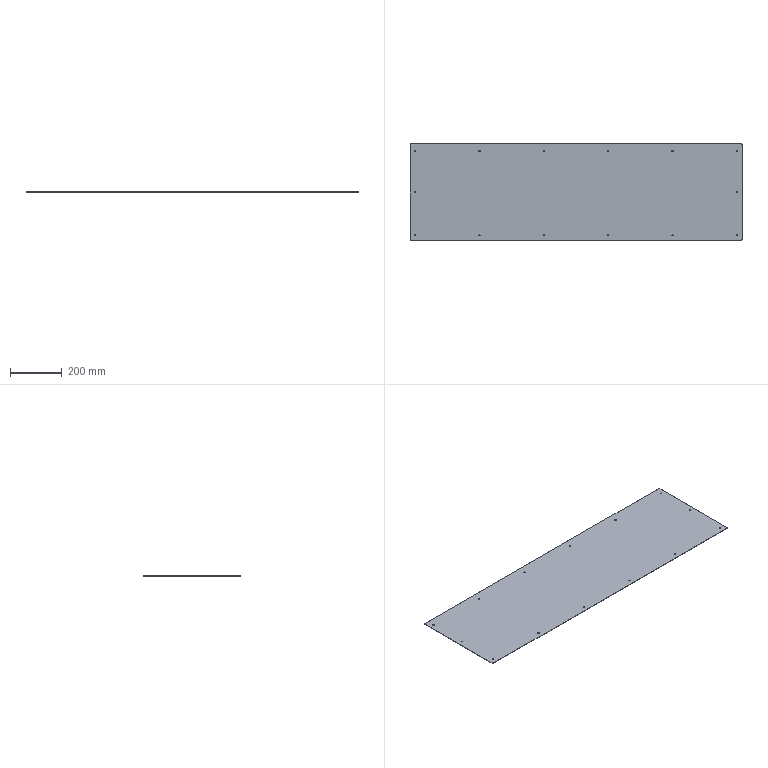Part | SolidWorks | features Fillet 1, FlatPattern 1, HoleWzd 1, SMBaseFlange 1, SheetMetal 1 | 1 solid | 38 faces | box 1280 x 374 x 1.5 mm | volume 717635 mm3 | cylinder 32 | plane 6 | commonest cylinder face diameters 5 x28 10 x4
STEP:
#1=CARTESIAN_POINT('',(-622.5,157.,-1.5));
#2=VERTEX_POINT('',#1);
#3=CARTESIAN_POINT('',(-617.5,157.,-1.5));
#4=VERTEX_POINT('',#3);
#5=CARTESIAN_POINT('',(-620.,157.,-1.5));
#6=DIRECTION('',(0.,0.,1.));
#7=DIRECTION('',(1.,0.,0.));
#8=AXIS2_PLACEMENT_3D('',#5,#6,#7);
#9=CIRCLE('',#8,2.5);
#10=EDGE_CURVE('',#2,#4,#9,.T.);
#11=ORIENTED_EDGE('',*,*,#10,.F.);
#12=CARTESIAN_POINT('',(-622.5,157.,0.));
#13=VERTEX_POINT('',#12);
#14=CARTESIAN_POINT('',(-622.5,157.,0.));
#15=DIRECTION('',(0.,0.,1.));
#16=VECTOR('',#15,1000.);
#17=LINE('',#14,#16);
#18=EDGE_CURVE('',#2,#13,#17,.T.);
#19=ORIENTED_EDGE('',*,*,#18,.T.);
#20=CARTESIAN_POINT('',(-617.5,157.,0.));
#21=VERTEX_POINT('',#20);
#22=CARTESIAN_POINT('',(-620.,157.,0.));
#23=DIRECTION('',(0.,0.,1.));
#24=DIRECTION('',(1.,0.,0.));
#25=AXIS2_PLACEMENT_3D('',#22,#23,#24);
#26=CIRCLE('',#25,2.5);
#27=EDGE_CURVE('',#13,#21,#26,.T.);
#28=ORIENTED_EDGE('',*,*,#27,.T.);
#29=CARTESIAN_POINT('',(-617.5,157.,0.));
#30=DIRECTION('',(0.,0.,1.));
#31=VECTOR('',#30,1000.);
#32=LINE('',#29,#31);
#33=EDGE_CURVE('',#4,#21,#32,.T.);
#34=ORIENTED_EDGE('',*,*,#33,.F.);
#35=EDGE_LOOP('',(#11,#19,#28,#34));
#36=FACE_OUTER_BOUND('',#35,.T.);
#37=CARTESIAN_POINT('',(-620.,157.,0.));
#38=DIRECTION('',(0.,0.,1.));
#39=DIRECTION('',(1.,0.,0.));
#40=AXIS2_PLACEMENT_3D('',#37,#38,#39);
#41=CYLINDRICAL_SURFACE('',#40,2.5);
#42=ADVANCED_FACE('',(#36),#41,.F.);
#43=CARTESIAN_POINT('',(617.5,157.,-1.5));
#44=VERTEX_POINT('',#43);
#45=CARTESIAN_POINT('',(622.5,157.,-1.5));
#46=VERTEX_POINT('',#45);
#47=CARTESIAN_POINT('',(620.,157.,-1.5));
#48=DIRECTION('',(0.,0.,1.));
#49=DIRECTION('',(1.,0.,0.));
#50=AXIS2_PLACEMENT_3D('',#47,#48,#49);
#51=CIRCLE('',#50,2.5);
#52=EDGE_CURVE('',#44,#46,#51,.T.);
#53=ORIENTED_EDGE('',*,*,#52,.F.);
#54=CARTESIAN_POINT('',(617.5,157.,0.));
#55=VERTEX_POINT('',#54);
#56=CARTESIAN_POINT('',(617.5,157.,0.));
#57=DIRECTION('',(0.,0.,1.));
#58=VECTOR('',#57,1000.);
#59=LINE('',#56,#58);
#60=EDGE_CURVE('',#44,#55,#59,.T.);
#61=ORIENTED_EDGE('',*,*,#60,.T.);
#62=CARTESIAN_POINT('',(622.5,157.,0.));
#63=VERTEX_POINT('',#62);
#64=CARTESIAN_POINT('',(620.,157.,0.));
#65=DIRECTION('',(0.,0.,1.));
#66=DIRECTION('',(1.,0.,0.));
#67=AXIS2_PLACEMENT_3D('',#64,#65,#66);
#68=CIRCLE('',#67,2.5);
#69=EDGE_CURVE('',#55,#63,#68,.T.);
#70=ORIENTED_EDGE('',*,*,#69,.T.);
#71=CARTESIAN_POINT('',(622.5,157.,0.));
#72=DIRECTION('',(0.,0.,1.));
#73=VECTOR('',#72,1000.);
#74=LINE('',#71,#73);
#75=EDGE_CURVE('',#46,#63,#74,.T.);
#76=ORIENTED_EDGE('',*,*,#75,.F.);
#77=EDGE_LOOP('',(#53,#61,#70,#76));
#78=FACE_OUTER_BOUND('',#77,.T.);
#79=CARTESIAN_POINT('',(620.,157.,0.));
#80=DIRECTION('',(0.,0.,1.));
#81=DIRECTION('',(1.,0.,0.));
#82=AXIS2_PLACEMENT_3D('',#79,#80,#81);
#83=CYLINDRICAL_SURFACE('',#82,2.5);
#84=ADVANCED_FACE('',(#78),#83,.F.);
#85=CARTESIAN_POINT('',(617.5,-167.,-1.5));
#86=VERTEX_POINT('',#85);
#87=CARTESIAN_POINT('',(622.5,-167.,-1.5));
#88=VERTEX_POINT('',#87);
#89=CARTESIAN_POINT('',(620.,-167.,-1.5));
#90=DIRECTION('',(0.,0.,1.));
#91=DIRECTION('',(1.,0.,0.));
#92=AXIS2_PLACEMENT_3D('',#89,#90,#91);
#93=CIRCLE('',#92,2.5);
#94=EDGE_CURVE('',#86,#88,#93,.T.);
#95=ORIENTED_EDGE('',*,*,#94,.F.);
#96=CARTESIAN_POINT('',(617.5,-167.,0.));
#97=VERTEX_POINT('',#96);
#98=CARTESIAN_POINT('',(617.5,-167.,0.));
#99=DIRECTION('',(0.,0.,1.));
#100=VECTOR('',#99,1000.);
#101=LINE('',#98,#100);
#102=EDGE_CURVE('',#86,#97,#101,.T.);
#103=ORIENTED_EDGE('',*,*,#102,.T.);
#104=CARTESIAN_POINT('',(622.5,-167.,0.));
#105=VERTEX_POINT('',#104);
#106=CARTESIAN_POINT('',(620.,-167.,0.));
#107=DIRECTION('',(0.,0.,1.));
#108=DIRECTION('',(1.,0.,0.));
#109=AXIS2_PLACEMENT_3D('',#106,#107,#108);
#110=CIRCLE('',#109,2.5);
#111=EDGE_CURVE('',#97,#105,#110,.T.);
#112=ORIENTED_EDGE('',*,*,#111,.T.);
#113=CARTESIAN_POINT('',(622.5,-167.,0.));
#114=DIRECTION('',(0.,0.,1.));
#115=VECTOR('',#114,1000.);
#116=LINE('',#113,#115);
#117=EDGE_CURVE('',#88,#105,#116,.T.);
#118=ORIENTED_EDGE('',*,*,#117,.F.);
#119=EDGE_LOOP('',(#95,#103,#112,#118));
#120=FACE_OUTER_BOUND('',#119,.T.);
#121=CARTESIAN_POINT('',(620.,-167.,0.));
#122=DIRECTION('',(0.,0.,1.));
#123=DIRECTION('',(1.,0.,0.));
#124=AXIS2_PLACEMENT_3D('',#121,#122,#123);
#125=CYLINDRICAL_SURFACE('',#124,2.5);
#126=ADVANCED_FACE('',(#120),#125,.F.);
#127=CARTESIAN_POINT('',(369.5,-167.,-1.5));
#128=VERTEX_POINT('',#127);
#129=CARTESIAN_POINT('',(374.5,-167.,-1.5));
#130=VERTEX_POINT('',#129);
#131=CARTESIAN_POINT('',(372.,-167.,-1.5));
#132=DIRECTION('',(0.,0.,1.));
#133=DIRECTION('',(1.,0.,0.));
#134=AXIS2_PLACEMENT_3D('',#131,#132,#133);
#135=CIRCLE('',#134,2.5);
#136=EDGE_CURVE('',#128,#130,#135,.T.);
#137=ORIENTED_EDGE('',*,*,#136,.F.);
#138=CARTESIAN_POINT('',(369.5,-167.,0.));
#139=VERTEX_POINT('',#138);
#140=CARTESIAN_POINT('',(369.5,-167.,0.));
#141=DIRECTION('',(0.,0.,1.));
#142=VECTOR('',#141,1000.);
#143=LINE('',#140,#142);
#144=EDGE_CURVE('',#128,#139,#143,.T.);
#145=ORIENTED_EDGE('',*,*,#144,.T.);
#146=CARTESIAN_POINT('',(374.5,-167.,0.));
#147=VERTEX_POINT('',#146);
#148=CARTESIAN_POINT('',(372.,-167.,0.));
#149=DIRECTION('',(0.,0.,1.));
#150=DIRECTION('',(1.,0.,0.));
#151=AXIS2_PLACEMENT_3D('',#148,#149,#150);
#152=CIRCLE('',#151,2.5);
#153=EDGE_CURVE('',#139,#147,#152,.T.);
#154=ORIENTED_EDGE('',*,*,#153,.T.);
#155=CARTESIAN_POINT('',(374.5,-167.,0.));
#156=DIRECTION('',(0.,0.,1.));
#157=VECTOR('',#156,1000.);
#158=LINE('',#155,#157);
#159=EDGE_CURVE('',#130,#147,#158,.T.);
#160=ORIENTED_EDGE('',*,*,#159,.F.);
#161=EDGE_LOOP('',(#137,#145,#154,#160));
#162=FACE_OUTER_BOUND('',#161,.T.);
#163=CARTESIAN_POINT('',(372.,-167.,0.));
#164=DIRECTION('',(0.,0.,1.));
#165=DIRECTION('',(1.,0.,0.));
#166=AXIS2_PLACEMENT_3D('',#163,#164,#165);
#167=CYLINDRICAL_SURFACE('',#166,2.5);
#168=ADVANCED_FACE('',(#162),#167,.F.);
#169=CARTESIAN_POINT('',(-374.5,-167.,-1.5));
#170=VERTEX_POINT('',#169);
#171=CARTESIAN_POINT('',(-369.5,-167.,-1.5));
#172=VERTEX_POINT('',#171);
#173=CARTESIAN_POINT('',(-372.,-167.,-1.5));
#174=DIRECTION('',(0.,0.,1.));
#175=DIRECTION('',(1.,0.,0.));
#176=AXIS2_PLACEMENT_3D('',#173,#174,#175);
#177=CIRCLE('',#176,2.5);
#178=EDGE_CURVE('',#170,#172,#177,.T.);
#179=ORIENTED_EDGE('',*,*,#178,.F.);
#180=CARTESIAN_POINT('',(-374.5,-167.,0.));
#181=VERTEX_POINT('',#180);
#182=CARTESIAN_POINT('',(-374.5,-167.,0.));
#183=DIRECTION('',(0.,0.,1.));
#184=VECTOR('',#183,1000.);
#185=LINE('',#182,#184);
#186=EDGE_CURVE('',#170,#181,#185,.T.);
#187=ORIENTED_EDGE('',*,*,#186,.T.);
#188=CARTESIAN_POINT('',(-369.5,-167.,0.));
#189=VERTEX_POINT('',#188);
#190=CARTESIAN_POINT('',(-372.,-167.,0.));
#191=DIRECTION('',(0.,0.,1.));
#192=DIRECTION('',(1.,0.,0.));
#193=AXIS2_PLACEMENT_3D('',#190,#191,#192);
#194=CIRCLE('',#193,2.5);
#195=EDGE_CURVE('',#181,#189,#194,.T.);
#196=ORIENTED_EDGE('',*,*,#195,.T.);
#197=CARTESIAN_POINT('',(-369.5,-167.,0.));
#198=DIRECTION('',(0.,0.,1.));
#199=VECTOR('',#198,1000.);
#200=LINE('',#197,#199);
#201=EDGE_CURVE('',#172,#189,#200,.T.);
#202=ORIENTED_EDGE('',*,*,#201,.F.);
#203=EDGE_LOOP('',(#179,#187,#196,#202));
#204=FACE_OUTER_BOUND('',#203,.T.);
#205=CARTESIAN_POINT('',(-372.,-167.,0.));
#206=DIRECTION('',(0.,0.,1.));
#207=DIRECTION('',(1.,0.,0.));
#208=AXIS2_PLACEMENT_3D('',#205,#206,#207);
#209=CYLINDRICAL_SURFACE('',#208,2.5);
#210=ADVANCED_FACE('',(#204),#209,.F.);
#211=CARTESIAN_POINT('',(-622.5,0.,-1.5));
#212=VERTEX_POINT('',#211);
#213=CARTESIAN_POINT('',(-617.5,0.,-1.5));
#214=VERTEX_POINT('',#213);
#215=CARTESIAN_POINT('',(-620.,0.,-1.5));
#216=DIRECTION('',(0.,0.,1.));
#217=DIRECTION('',(1.,0.,0.));
#218=AXIS2_PLACEMENT_3D('',#215,#216,#217);
#219=CIRCLE('',#218,2.5);
#220=EDGE_CURVE('',#212,#214,#219,.T.);
#221=ORIENTED_EDGE('',*,*,#220,.F.);
#222=CARTESIAN_POINT('',(-622.5,0.,0.));
#223=VERTEX_POINT('',#222);
#224=CARTESIAN_POINT('',(-622.5,0.,0.));
#225=DIRECTION('',(0.,0.,1.));
#226=VECTOR('',#225,1000.);
#227=LINE('',#224,#226);
#228=EDGE_CURVE('',#212,#223,#227,.T.);
#229=ORIENTED_EDGE('',*,*,#228,.T.);
#230=CARTESIAN_POINT('',(-617.5,0.,0.));
#231=VERTEX_POINT('',#230);
#232=CARTESIAN_POINT('',(-620.,0.,0.));
#233=DIRECTION('',(0.,0.,1.));
#234=DIRECTION('',(1.,0.,0.));
#235=AXIS2_PLACEMENT_3D('',#232,#233,#234);
#236=CIRCLE('',#235,2.5);
#237=EDGE_CURVE('',#223,#231,#236,.T.);
#238=ORIENTED_EDGE('',*,*,#237,.T.);
#239=CARTESIAN_POINT('',(-617.5,0.,0.));
#240=DIRECTION('',(0.,0.,1.));
#241=VECTOR('',#240,1000.);
#242=LINE('',#239,#241);
#243=EDGE_CURVE('',#214,#231,#242,.T.);
#244=ORIENTED_EDGE('',*,*,#243,.F.);
#245=EDGE_LOOP('',(#221,#229,#238,#244));
#246=FACE_OUTER_BOUND('',#245,.T.);
#247=CARTESIAN_POINT('',(-620.,0.,0.));
#248=DIRECTION('',(0.,0.,1.));
#249=DIRECTION('',(1.,0.,0.));
#250=AXIS2_PLACEMENT_3D('',#247,#248,#249);
#251=CYLINDRICAL_SURFACE('',#250,2.5);
#252=ADVANCED_FACE('',(#246),#251,.F.);
#253=CARTESIAN_POINT('',(-622.5,-167.,-1.5));
#254=VERTEX_POINT('',#253);
#255=CARTESIAN_POINT('',(-617.5,-167.,-1.5));
#256=VERTEX_POINT('',#255);
#257=CARTESIAN_POINT('',(-620.,-167.,-1.5));
#258=DIRECTION('',(0.,0.,1.));
#259=DIRECTION('',(1.,0.,0.));
#260=AXIS2_PLACEMENT_3D('',#257,#258,#259);
#261=CIRCLE('',#260,2.5);
#262=EDGE_CURVE('',#254,#256,#261,.T.);
#263=ORIENTED_EDGE('',*,*,#262,.F.);
#264=CARTESIAN_POINT('',(-622.5,-167.,0.));
#265=VERTEX_POINT('',#264);
#266=CARTESIAN_POINT('',(-622.5,-167.,0.));
#267=DIRECTION('',(0.,0.,1.));
#268=VECTOR('',#267,1000.);
#269=LINE('',#266,#268);
#270=EDGE_CURVE('',#254,#265,#269,.T.);
#271=ORIENTED_EDGE('',*,*,#270,.T.);
#272=CARTESIAN_POINT('',(-617.5,-167.,0.));
#273=VERTEX_POINT('',#272);
#274=CARTESIAN_POINT('',(-620.,-167.,0.));
#275=DIRECTION('',(0.,0.,1.));
#276=DIRECTION('',(1.,0.,0.));
#277=AXIS2_PLACEMENT_3D('',#274,#275,#276);
#278=CIRCLE('',#277,2.5);
#279=EDGE_CURVE('',#265,#273,#278,.T.);
#280=ORIENTED_EDGE('',*,*,#279,.T.);
#281=CARTESIAN_POINT('',(-617.5,-167.,0.));
#282=DIRECTION('',(0.,0.,1.));
#283=VECTOR('',#282,1000.);
#284=LINE('',#281,#283);
#285=EDGE_CURVE('',#256,#273,#284,.T.);
#286=ORIENTED_EDGE('',*,*,#285,.F.);
#287=EDGE_LOOP('',(#263,#271,#280,#286));
#288=FACE_OUTER_BOUND('',#287,.T.);
#289=CARTESIAN_POINT('',(-620.,-167.,0.));
#290=DIRECTION('',(0.,0.,1.));
#291=DIRECTION('',(1.,0.,0.));
#292=AXIS2_PLACEMENT_3D('',#289,#290,#291);
#293=CYLINDRICAL_SURFACE('',#292,2.5);
#294=ADVANCED_FACE('',(#288),#293,.F.);
#295=CARTESIAN_POINT('',(617.5,0.,-1.5));
#296=VERTEX_POINT('',#295);
#297=CARTESIAN_POINT('',(622.5,0.,-1.5));
#298=VERTEX_POINT('',#297);
#299=CARTESIAN_POINT('',(620.,0.,-1.5));
#300=DIRECTION('',(0.,0.,1.));
#301=DIRECTION('',(1.,0.,0.));
#302=AXIS2_PLACEMENT_3D('',#299,#300,#301);
#303=CIRCLE('',#302,2.5);
#304=EDGE_CURVE('',#296,#298,#303,.T.);
#305=ORIENTED_EDGE('',*,*,#304,.F.);
#306=CARTESIAN_POINT('',(617.5,0.,0.));
#307=VERTEX_POINT('',#306);
#308=CARTESIAN_POINT('',(617.5,0.,0.));
#309=DIRECTION('',(0.,0.,1.));
#310=VECTOR('',#309,1000.);
#311=LINE('',#308,#310);
#312=EDGE_CURVE('',#296,#307,#311,.T.);
#313=ORIENTED_EDGE('',*,*,#312,.T.);
#314=CARTESIAN_POINT('',(622.5,0.,0.));
#315=VERTEX_POINT('',#314);
#316=CARTESIAN_POINT('',(620.,0.,0.));
#317=DIRECTION('',(0.,0.,1.));
#318=DIRECTION('',(1.,0.,0.));
#319=AXIS2_PLACEMENT_3D('',#316,#317,#318);
#320=CIRCLE('',#319,2.5);
#321=EDGE_CURVE('',#307,#315,#320,.T.);
#322=ORIENTED_EDGE('',*,*,#321,.T.);
#323=CARTESIAN_POINT('',(622.5,0.,0.));
#324=DIRECTION('',(0.,0.,1.));
#325=VECTOR('',#324,1000.);
#326=LINE('',#323,#325);
#327=EDGE_CURVE('',#298,#315,#326,.T.);
#328=ORIENTED_EDGE('',*,*,#327,.F.);
#329=EDGE_LOOP('',(#305,#313,#322,#328));
#330=FACE_OUTER_BOUND('',#329,.T.);
#331=CARTESIAN_POINT('',(620.,0.,0.));
#332=DIRECTION('',(0.,0.,1.));
#333=DIRECTION('',(1.,0.,0.));
#334=AXIS2_PLACEMENT_3D('',#331,#332,#333);
#335=CYLINDRICAL_SURFACE('',#334,2.5);
#336=ADVANCED_FACE('',(#330),#335,.F.);
#337=CARTESIAN_POINT('',(-126.5,-167.,-1.5));
#338=VERTEX_POINT('',#337);
#339=CARTESIAN_POINT('',(-121.5,-167.,-1.5));
#340=VERTEX_POINT('',#339);
#341=CARTESIAN_POINT('',(-124.,-167.,-1.5));
#342=DIRECTION('',(0.,0.,1.));
#343=DIRECTION('',(1.,0.,0.));
#344=AXIS2_PLACEMENT_3D('',#341,#342,#343);
#345=CIRCLE('',#344,2.5);
#346=EDGE_CURVE('',#338,#340,#345,.T.);
#347=ORIENTED_EDGE('',*,*,#346,.F.);
#348=CARTESIAN_POINT('',(-126.5,-167.,0.));
#349=VERTEX_POINT('',#348);
#350=CARTESIAN_POINT('',(-126.5,-167.,0.));
#351=DIRECTION('',(0.,0.,1.));
#352=VECTOR('',#351,1000.);
#353=LINE('',#350,#352);
#354=EDGE_CURVE('',#338,#349,#353,.T.);
#355=ORIENTED_EDGE('',*,*,#354,.T.);
#356=CARTESIAN_POINT('',(-121.5,-167.,0.));
#357=VERTEX_POINT('',#356);
#358=CARTESIAN_POINT('',(-124.,-167.,0.));
#359=DIRECTION('',(0.,0.,1.));
#360=DIRECTION('',(1.,0.,0.));
#361=AXIS2_PLACEMENT_3D('',#358,#359,#360);
#362=CIRCLE('',#361,2.5);
#363=EDGE_CURVE('',#349,#357,#362,.T.);
#364=ORIENTED_EDGE('',*,*,#363,.T.);
#365=CARTESIAN_POINT('',(-121.5,-167.,0.));
#366=DIRECTION('',(0.,0.,1.));
#367=VECTOR('',#366,1000.);
#368=LINE('',#365,#367);
#369=EDGE_CURVE('',#340,#357,#368,.T.);
#370=ORIENTED_EDGE('',*,*,#369,.F.);
#371=EDGE_LOOP('',(#347,#355,#364,#370));
#372=FACE_OUTER_BOUND('',#371,.T.);
#373=CARTESIAN_POINT('',(-124.,-167.,0.));
#374=DIRECTION('',(0.,0.,1.));
#375=DIRECTION('',(1.,0.,0.));
#376=AXIS2_PLACEMENT_3D('',#373,#374,#375);
#377=CYLINDRICAL_SURFACE('',#376,2.5);
#378=ADVANCED_FACE('',(#372),#377,.F.);
#379=CARTESIAN_POINT('',(121.5,-167.,-1.5));
#380=VERTEX_POINT('',#379);
#381=CARTESIAN_POINT('',(126.5,-167.,-1.5));
#382=VERTEX_POINT('',#381);
#383=CARTESIAN_POINT('',(124.,-167.,-1.5));
#384=DIRECTION('',(0.,0.,1.));
#385=DIRECTION('',(1.,0.,0.));
#386=AXIS2_PLACEMENT_3D('',#383,#384,#385);
#387=CIRCLE('',#386,2.5);
#388=EDGE_CURVE('',#380,#382,#387,.T.);
#389=ORIENTED_EDGE('',*,*,#388,.F.);
#390=CARTESIAN_POINT('',(121.5,-167.,0.));
#391=VERTEX_POINT('',#390);
#392=CARTESIAN_POINT('',(121.5,-167.,0.));
#393=DIRECTION('',(0.,0.,1.));
#394=VECTOR('',#393,1000.);
#395=LINE('',#392,#394);
#396=EDGE_CURVE('',#380,#391,#395,.T.);
#397=ORIENTED_EDGE('',*,*,#396,.T.);
#398=CARTESIAN_POINT('',(126.5,-167.,0.));
#399=VERTEX_POINT('',#398);
#400=CARTESIAN_POINT('',(124.,-167.,0.));
#401=DIRECTION('',(0.,0.,1.));
#402=DIRECTION('',(1.,0.,0.));
#403=AXIS2_PLACEMENT_3D('',#400,#401,#402);
#404=CIRCLE('',#403,2.5);
#405=EDGE_CURVE('',#391,#399,#404,.T.);
#406=ORIENTED_EDGE('',*,*,#405,.T.);
#407=CARTESIAN_POINT('',(126.5,-167.,0.));
#408=DIRECTION('',(0.,0.,1.));
#409=VECTOR('',#408,1000.);
#410=LINE('',#407,#409);
#411=EDGE_CURVE('',#382,#399,#410,.T.);
#412=ORIENTED_EDGE('',*,*,#411,.F.);
#413=EDGE_LOOP('',(#389,#397,#406,#412));
#414=FACE_OUTER_BOUND('',#413,.T.);
#415=CARTESIAN_POINT('',(124.,-167.,0.));
#416=DIRECTION('',(0.,0.,1.));
#417=DIRECTION('',(1.,0.,0.));
#418=AXIS2_PLACEMENT_3D('',#415,#416,#417);
#419=CYLINDRICAL_SURFACE('',#418,2.5);
#420=ADVANCED_FACE('',(#414),#419,.F.);
#421=CARTESIAN_POINT('',(-126.5,157.,-1.5));
#422=VERTEX_POINT('',#421);
#423=CARTESIAN_POINT('',(-121.5,157.,-1.5));
#424=VERTEX_POINT('',#423);
#425=CARTESIAN_POINT('',(-124.,157.,-1.5));
#426=DIRECTION('',(0.,0.,1.));
#427=DIRECTION('',(1.,0.,0.));
#428=AXIS2_PLACEMENT_3D('',#425,#426,#427);
#429=CIRCLE('',#428,2.5);
#430=EDGE_CURVE('',#422,#424,#429,.T.);
#431=ORIENTED_EDGE('',*,*,#430,.F.);
#432=CARTESIAN_POINT('',(-126.5,157.,0.));
#433=VERTEX_POINT('',#432);
#434=CARTESIAN_POINT('',(-126.5,157.,0.));
#435=DIRECTION('',(0.,0.,1.));
#436=VECTOR('',#435,1000.);
#437=LINE('',#434,#436);
#438=EDGE_CURVE('',#422,#433,#437,.T.);
#439=ORIENTED_EDGE('',*,*,#438,.T.);
#440=CARTESIAN_POINT('',(-121.5,157.,0.));
#441=VERTEX_POINT('',#440);
#442=CARTESIAN_POINT('',(-124.,157.,0.));
#443=DIRECTION('',(0.,0.,1.));
#444=DIRECTION('',(1.,0.,0.));
#445=AXIS2_PLACEMENT_3D('',#442,#443,#444);
#446=CIRCLE('',#445,2.5);
#447=EDGE_CURVE('',#433,#441,#446,.T.);
#448=ORIENTED_EDGE('',*,*,#447,.T.);
#449=CARTESIAN_POINT('',(-121.5,157.,0.));
#450=DIRECTION('',(0.,0.,1.));
#451=VECTOR('',#450,1000.);
#452=LINE('',#449,#451);
#453=EDGE_CURVE('',#424,#441,#452,.T.);
#454=ORIENTED_EDGE('',*,*,#453,.F.);
#455=EDGE_LOOP('',(#431,#439,#448,#454));
#456=FACE_OUTER_BOUND('',#455,.T.);
#457=CARTESIAN_POINT('',(-124.,157.,0.));
#458=DIRECTION('',(0.,0.,1.));
#459=DIRECTION('',(1.,0.,0.));
#460=AXIS2_PLACEMENT_3D('',#457,#458,#459);
#461=CYLINDRICAL_SURFACE('',#460,2.5);
#462=ADVANCED_FACE('',(#456),#461,.F.);
#463=CARTESIAN_POINT('',(121.5,157.,-1.5));
#464=VERTEX_POINT('',#463);
#465=CARTESIAN_POINT('',(126.5,157.,-1.5));
#466=VERTEX_POINT('',#465);
#467=CARTESIAN_POINT('',(124.,157.,-1.5));
#468=DIRECTION('',(0.,0.,1.));
#469=DIRECTION('',(1.,0.,0.));
#470=AXIS2_PLACEMENT_3D('',#467,#468,#469);
#471=CIRCLE('',#470,2.5);
#472=EDGE_CURVE('',#464,#466,#471,.T.);
#473=ORIENTED_EDGE('',*,*,#472,.F.);
#474=CARTESIAN_POINT('',(121.5,157.,0.));
#475=VERTEX_POINT('',#474);
#476=CARTESIAN_POINT('',(121.5,157.,0.));
#477=DIRECTION('',(0.,0.,1.));
#478=VECTOR('',#477,1000.);
#479=LINE('',#476,#478);
#480=EDGE_CURVE('',#464,#475,#479,.T.);
#481=ORIENTED_EDGE('',*,*,#480,.T.);
#482=CARTESIAN_POINT('',(126.5,157.,0.));
#483=VERTEX_POINT('',#482);
#484=CARTESIAN_POINT('',(124.,157.,0.));
#485=DIRECTION('',(0.,0.,1.));
#486=DIRECTION('',(1.,0.,0.));
#487=AXIS2_PLACEMENT_3D('',#484,#485,#486);
#488=CIRCLE('',#487,2.5);
#489=EDGE_CURVE('',#475,#483,#488,.T.);
#490=ORIENTED_EDGE('',*,*,#489,.T.);
#491=CARTESIAN_POINT('',(126.5,157.,0.));
#492=DIRECTION('',(0.,0.,1.));
#493=VECTOR('',#492,1000.);
#494=LINE('',#491,#493);
#495=EDGE_CURVE('',#466,#483,#494,.T.);
#496=ORIENTED_EDGE('',*,*,#495,.F.);
#497=EDGE_LOOP('',(#473,#481,#490,#496));
#498=FACE_OUTER_BOUND('',#497,.T.);
#499=CARTESIAN_POINT('',(124.,157.,0.));
#500=DIRECTION('',(0.,0.,1.));
#501=DIRECTION('',(1.,0.,0.));
#502=AXIS2_PLACEMENT_3D('',#499,#500,#501);
#503=CYLINDRICAL_SURFACE('',#502,2.5);
#504=ADVANCED_FACE('',(#498),#503,.F.);
#505=CARTESIAN_POINT('',(369.5,157.,-1.5));
#506=VERTEX_POINT('',#505);
#507=CARTESIAN_POINT('',(374.5,157.,-1.5));
#508=VERTEX_POINT('',#507);
#509=CARTESIAN_POINT('',(372.,157.,-1.5));
#510=DIRECTION('',(0.,0.,1.));
#511=DIRECTION('',(1.,0.,0.));
#512=AXIS2_PLACEMENT_3D('',#509,#510,#511);
#513=CIRCLE('',#512,2.5);
#514=EDGE_CURVE('',#506,#508,#513,.T.);
#515=ORIENTED_EDGE('',*,*,#514,.F.);
#516=CARTESIAN_POINT('',(369.5,157.,0.));
#517=VERTEX_POINT('',#516);
#518=CARTESIAN_POINT('',(369.5,157.,0.));
#519=DIRECTION('',(0.,0.,1.));
#520=VECTOR('',#519,1000.);
#521=LINE('',#518,#520);
#522=EDGE_CURVE('',#506,#517,#521,.T.);
#523=ORIENTED_EDGE('',*,*,#522,.T.);
#524=CARTESIAN_POINT('',(374.5,157.,0.));
#525=VERTEX_POINT('',#524);
#526=CARTESIAN_POINT('',(372.,157.,0.));
#527=DIRECTION('',(0.,0.,1.));
#528=DIRECTION('',(1.,0.,0.));
#529=AXIS2_PLACEMENT_3D('',#526,#527,#528);
#530=CIRCLE('',#529,2.5);
#531=EDGE_CURVE('',#517,#525,#530,.T.);
#532=ORIENTED_EDGE('',*,*,#531,.T.);
#533=CARTESIAN_POINT('',(374.5,157.,0.));
#534=DIRECTION('',(0.,0.,1.));
#535=VECTOR('',#534,1000.);
#536=LINE('',#533,#535);
#537=EDGE_CURVE('',#508,#525,#536,.T.);
#538=ORIENTED_EDGE('',*,*,#537,.F.);
#539=EDGE_LOOP('',(#515,#523,#532,#538));
#540=FACE_OUTER_BOUND('',#539,.T.);
#541=CARTESIAN_POINT('',(372.,157.,0.));
#542=DIRECTION('',(0.,0.,1.));
#543=DIRECTION('',(1.,0.,0.));
#544=AXIS2_PLACEMENT_3D('',#541,#542,#543);
#545=CYLINDRICAL_SURFACE('',#544,2.5);
#546=ADVANCED_FACE('',(#540),#545,.F.);
#547=CARTESIAN_POINT('',(-374.5,157.,-1.5));
#548=VERTEX_POINT('',#547);
#549=CARTESIAN_POINT('',(-369.5,157.,-1.5));
#550=VERTEX_POINT('',#549);
#551=CARTESIAN_POINT('',(-372.,157.,-1.5));
#552=DIRECTION('',(0.,0.,1.));
#553=DIRECTION('',(1.,0.,0.));
#554=AXIS2_PLACEMENT_3D('',#551,#552,#553);
#555=CIRCLE('',#554,2.5);
#556=EDGE_CURVE('',#548,#550,#555,.T.);
#557=ORIENTED_EDGE('',*,*,#556,.F.);
#558=CARTESIAN_POINT('',(-374.5,157.,0.));
#559=VERTEX_POINT('',#558);
#560=CARTESIAN_POINT('',(-374.5,157.,0.));
#561=DIRECTION('',(0.,0.,1.));
#562=VECTOR('',#561,1000.);
#563=LINE('',#560,#562);
#564=EDGE_CURVE('',#548,#559,#563,.T.);
#565=ORIENTED_EDGE('',*,*,#564,.T.);
#566=CARTESIAN_POINT('',(-369.5,157.,0.));
#567=VERTEX_POINT('',#566);
#568=CARTESIAN_POINT('',(-372.,157.,0.));
#569=DIRECTION('',(0.,0.,1.));
#570=DIRECTION('',(1.,0.,0.));
#571=AXIS2_PLACEMENT_3D('',#568,#569,#570);
#572=CIRCLE('',#571,2.5);
#573=EDGE_CURVE('',#559,#567,#572,.T.);
#574=ORIENTED_EDGE('',*,*,#573,.T.);
#575=CARTESIAN_POINT('',(-369.5,157.,0.));
#576=DIRECTION('',(0.,0.,1.));
#577=VECTOR('',#576,1000.);
#578=LINE('',#575,#577);
#579=EDGE_CURVE('',#550,#567,#578,.T.);
#580=ORIENTED_EDGE('',*,*,#579,.F.);
#581=EDGE_LOOP('',(#557,#565,#574,#580));
#582=FACE_OUTER_BOUND('',#581,.T.);
#583=CARTESIAN_POINT('',(-372.,157.,0.));
#584=DIRECTION('',(0.,0.,1.));
#585=DIRECTION('',(1.,0.,0.));
#586=AXIS2_PLACEMENT_3D('',#583,#584,#585);
#587=CYLINDRICAL_SURFACE('',#586,2.5);
#588=ADVANCED_FACE('',(#582),#587,.F.);
#589=CARTESIAN_POINT('',(640.,-182.,0.));
#590=VERTEX_POINT('',#589);
#591=CARTESIAN_POINT('',(640.,182.,0.));
#592=VERTEX_POINT('',#591);
#593=CARTESIAN_POINT('',(640.,187.,0.));
#594=DIRECTION('',(0.,1.,0.));
#595=VECTOR('',#594,1000.);
#596=LINE('',#593,#595);
#597=EDGE_CURVE('',#590,#592,#596,.T.);
#598=ORIENTED_EDGE('',*,*,#597,.F.);
#599=CARTESIAN_POINT('',(640.,-182.,-1.5));
#600=VERTEX_POINT('',#599);
#601=CARTESIAN_POINT('',(640.,-182.,-1.5));
#602=DIRECTION('',(0.,0.,-1.));
#603=VECTOR('',#602,1000.);
#604=LINE('',#601,#603);
#605=EDGE_CURVE('',#590,#600,#604,.T.);
#606=ORIENTED_EDGE('',*,*,#605,.T.);
#607=CARTESIAN_POINT('',(640.,182.,-1.5));
#608=VERTEX_POINT('',#607);
#609=CARTESIAN_POINT('',(640.,187.,-1.5));
#610=DIRECTION('',(0.,1.,0.));
#611=VECTOR('',#610,1000.);
#612=LINE('',#609,#611);
#613=EDGE_CURVE('',#600,#608,#612,.T.);
#614=ORIENTED_EDGE('',*,*,#613,.T.);
#615=CARTESIAN_POINT('',(640.,182.,-1.5));
#616=DIRECTION('',(0.,0.,1.));
#617=VECTOR('',#616,1000.);
#618=LINE('',#615,#617);
#619=EDGE_CURVE('',#608,#592,#618,.T.);
#620=ORIENTED_EDGE('',*,*,#619,.T.);
#621=EDGE_LOOP('',(#598,#606,#614,#620));
#622=FACE_OUTER_BOUND('',#621,.T.);
#623=CARTESIAN_POINT('',(640.,187.,-1.5));
#624=DIRECTION('',(1.,0.,0.));
#625=DIRECTION('',(0.,0.,-1.));
#626=AXIS2_PLACEMENT_3D('',#623,#624,#625);
#627=PLANE('',#626);
#628=ADVANCED_FACE('',(#622),#627,.T.);
#629=CARTESIAN_POINT('',(-635.,-187.,0.));
#630=VERTEX_POINT('',#629);
#631=CARTESIAN_POINT('',(635.,-187.,0.));
#632=VERTEX_POINT('',#631);
#633=CARTESIAN_POINT('',(-640.,-187.,0.));
#634=DIRECTION('',(1.,0.,0.));
#635=VECTOR('',#634,1000.);
#636=LINE('',#633,#635);
#637=EDGE_CURVE('',#630,#632,#636,.T.);
#638=ORIENTED_EDGE('',*,*,#637,.F.);
#639=CARTESIAN_POINT('',(-635.,-187.,-1.5));
#640=VERTEX_POINT('',#639);
#641=CARTESIAN_POINT('',(-635.,-187.,-1.5));
#642=DIRECTION('',(0.,0.,-1.));
#643=VECTOR('',#642,1000.);
#644=LINE('',#641,#643);
#645=EDGE_CURVE('',#630,#640,#644,.T.);
#646=ORIENTED_EDGE('',*,*,#645,.T.);
#647=CARTESIAN_POINT('',(635.,-187.,-1.5));
#648=VERTEX_POINT('',#647);
#649=CARTESIAN_POINT('',(-640.,-187.,-1.5));
#650=DIRECTION('',(1.,0.,0.));
#651=VECTOR('',#650,1000.);
#652=LINE('',#649,#651);
#653=EDGE_CURVE('',#640,#648,#652,.T.);
#654=ORIENTED_EDGE('',*,*,#653,.T.);
#655=CARTESIAN_POINT('',(635.,-187.,-1.5));
#656=DIRECTION('',(0.,0.,1.));
#657=VECTOR('',#656,1000.);
#658=LINE('',#655,#657);
#659=EDGE_CURVE('',#648,#632,#658,.T.);
#660=ORIENTED_EDGE('',*,*,#659,.T.);
#661=EDGE_LOOP('',(#638,#646,#654,#660));
#662=FACE_OUTER_BOUND('',#661,.T.);
#663=CARTESIAN_POINT('',(-640.,-187.,-1.5));
#664=DIRECTION('',(0.,-1.,0.));
#665=DIRECTION('',(0.,0.,-1.));
#666=AXIS2_PLACEMENT_3D('',#663,#664,#665);
#667=PLANE('',#666);
#668=ADVANCED_FACE('',(#662),#667,.T.);
#669=CARTESIAN_POINT('',(-640.,182.,-1.5));
#670=VERTEX_POINT('',#669);
#671=CARTESIAN_POINT('',(-640.,-182.,-1.5));
#672=VERTEX_POINT('',#671);
#673=CARTESIAN_POINT('',(-640.,187.,-1.5));
#674=DIRECTION('',(0.,-1.,0.));
#675=VECTOR('',#674,1000.);
#676=LINE('',#673,#675);
#677=EDGE_CURVE('',#670,#672,#676,.T.);
#678=ORIENTED_EDGE('',*,*,#677,.T.);
#679=CARTESIAN_POINT('',(-640.,-182.,0.));
#680=VERTEX_POINT('',#679);
#681=CARTESIAN_POINT('',(-640.,-182.,-1.5));
#682=DIRECTION('',(0.,0.,1.));
#683=VECTOR('',#682,1000.);
#684=LINE('',#681,#683);
#685=EDGE_CURVE('',#672,#680,#684,.T.);
#686=ORIENTED_EDGE('',*,*,#685,.T.);
#687=CARTESIAN_POINT('',(-640.,182.,0.));
#688=VERTEX_POINT('',#687);
#689=CARTESIAN_POINT('',(-640.,187.,0.));
#690=DIRECTION('',(0.,-1.,0.));
#691=VECTOR('',#690,1000.);
#692=LINE('',#689,#691);
#693=EDGE_CURVE('',#688,#680,#692,.T.);
#694=ORIENTED_EDGE('',*,*,#693,.F.);
#695=CARTESIAN_POINT('',(-640.,182.,-1.5));
#696=DIRECTION('',(0.,0.,-1.));
#697=VECTOR('',#696,1000.);
#698=LINE('',#695,#697);
#699=EDGE_CURVE('',#688,#670,#698,.T.);
#700=ORIENTED_EDGE('',*,*,#699,.T.);
#701=EDGE_LOOP('',(#678,#686,#694,#700));
#702=FACE_OUTER_BOUND('',#701,.T.);
#703=CARTESIAN_POINT('',(-640.,187.,-1.5));
#704=DIRECTION('',(-1.,0.,0.));
#705=DIRECTION('',(0.,0.,1.));
#706=AXIS2_PLACEMENT_3D('',#703,#704,#705);
#707=PLANE('',#706);
#708=ADVANCED_FACE('',(#702),#707,.T.);
#709=CARTESIAN_POINT('',(635.,187.,0.));
#710=VERTEX_POINT('',#709);
#711=CARTESIAN_POINT('',(-635.,187.,0.));
#712=VERTEX_POINT('',#711);
#713=CARTESIAN_POINT('',(-640.,187.,0.));
#714=DIRECTION('',(-1.,0.,0.));
#715=VECTOR('',#714,1000.);
#716=LINE('',#713,#715);
#717=EDGE_CURVE('',#710,#712,#716,.T.);
#718=ORIENTED_EDGE('',*,*,#717,.F.);
#719=CARTESIAN_POINT('',(635.,187.,-1.5));
#720=VERTEX_POINT('',#719);
#721=CARTESIAN_POINT('',(635.,187.,-1.5));
#722=DIRECTION('',(0.,0.,-1.));
#723=VECTOR('',#722,1000.);
#724=LINE('',#721,#723);
#725=EDGE_CURVE('',#710,#720,#724,.T.);
#726=ORIENTED_EDGE('',*,*,#725,.T.);
#727=CARTESIAN_POINT('',(-635.,187.,-1.5));
#728=VERTEX_POINT('',#727);
#729=CARTESIAN_POINT('',(-640.,187.,-1.5));
#730=DIRECTION('',(-1.,0.,0.));
#731=VECTOR('',#730,1000.);
#732=LINE('',#729,#731);
#733=EDGE_CURVE('',#720,#728,#732,.T.);
#734=ORIENTED_EDGE('',*,*,#733,.T.);
#735=CARTESIAN_POINT('',(-635.,187.,-1.5));
#736=DIRECTION('',(0.,0.,1.));
#737=VECTOR('',#736,1000.);
#738=LINE('',#735,#737);
#739=EDGE_CURVE('',#728,#712,#738,.T.);
#740=ORIENTED_EDGE('',*,*,#739,.T.);
#741=EDGE_LOOP('',(#718,#726,#734,#740));
#742=FACE_OUTER_BOUND('',#741,.T.);
#743=CARTESIAN_POINT('',(-640.,187.,-1.5));
#744=DIRECTION('',(0.,1.,0.));
#745=DIRECTION('',(0.,0.,1.));
#746=AXIS2_PLACEMENT_3D('',#743,#744,#745);
#747=PLANE('',#746);
#748=ADVANCED_FACE('',(#742),#747,.T.);
#749=CARTESIAN_POINT('',(-620.,157.,-1.5));
#750=DIRECTION('',(0.,0.,1.));
#751=DIRECTION('',(1.,0.,0.));
#752=AXIS2_PLACEMENT_3D('',#749,#750,#751);
#753=CIRCLE('',#752,2.5);
#754=EDGE_CURVE('',#4,#2,#753,.T.);
#755=ORIENTED_EDGE('',*,*,#754,.T.);
#756=ORIENTED_EDGE('',*,*,#10,.T.);
#757=EDGE_LOOP('',(#755,#756));
#758=FACE_BOUND('',#757,.T.);
#759=CARTESIAN_POINT('',(620.,157.,-1.5));
#760=DIRECTION('',(0.,0.,1.));
#761=DIRECTION('',(1.,0.,0.));
#762=AXIS2_PLACEMENT_3D('',#759,#760,#761);
#763=CIRCLE('',#762,2.5);
#764=EDGE_CURVE('',#46,#44,#763,.T.);
#765=ORIENTED_EDGE('',*,*,#764,.T.);
#766=ORIENTED_EDGE('',*,*,#52,.T.);
#767=EDGE_LOOP('',(#765,#766));
#768=FACE_BOUND('',#767,.T.);
#769=CARTESIAN_POINT('',(620.,-167.,-1.5));
#770=DIRECTION('',(0.,0.,1.));
#771=DIRECTION('',(1.,0.,0.));
#772=AXIS2_PLACEMENT_3D('',#769,#770,#771);
#773=CIRCLE('',#772,2.5);
#774=EDGE_CURVE('',#88,#86,#773,.T.);
#775=ORIENTED_EDGE('',*,*,#774,.T.);
#776=ORIENTED_EDGE('',*,*,#94,.T.);
#777=EDGE_LOOP('',(#775,#776));
#778=FACE_BOUND('',#777,.T.);
#779=CARTESIAN_POINT('',(372.,-167.,-1.5));
#780=DIRECTION('',(0.,0.,1.));
#781=DIRECTION('',(1.,0.,0.));
#782=AXIS2_PLACEMENT_3D('',#779,#780,#781);
#783=CIRCLE('',#782,2.5);
#784=EDGE_CURVE('',#130,#128,#783,.T.);
#785=ORIENTED_EDGE('',*,*,#784,.T.);
#786=ORIENTED_EDGE('',*,*,#136,.T.);
#787=EDGE_LOOP('',(#785,#786));
#788=FACE_BOUND('',#787,.T.);
#789=CARTESIAN_POINT('',(-372.,-167.,-1.5));
#790=DIRECTION('',(0.,0.,1.));
#791=DIRECTION('',(1.,0.,0.));
#792=AXIS2_PLACEMENT_3D('',#789,#790,#791);
#793=CIRCLE('',#792,2.5);
#794=EDGE_CURVE('',#172,#170,#793,.T.);
#795=ORIENTED_EDGE('',*,*,#794,.T.);
#796=ORIENTED_EDGE('',*,*,#178,.T.);
#797=EDGE_LOOP('',(#795,#796));
#798=FACE_BOUND('',#797,.T.);
#799=CARTESIAN_POINT('',(-620.,0.,-1.5));
#800=DIRECTION('',(0.,0.,1.));
#801=DIRECTION('',(1.,0.,0.));
#802=AXIS2_PLACEMENT_3D('',#799,#800,#801);
#803=CIRCLE('',#802,2.5);
#804=EDGE_CURVE('',#214,#212,#803,.T.);
#805=ORIENTED_EDGE('',*,*,#804,.T.);
#806=ORIENTED_EDGE('',*,*,#220,.T.);
#807=EDGE_LOOP('',(#805,#806));
#808=FACE_BOUND('',#807,.T.);
#809=CARTESIAN_POINT('',(-620.,-167.,-1.5));
#810=DIRECTION('',(0.,0.,1.));
#811=DIRECTION('',(1.,0.,0.));
#812=AXIS2_PLACEMENT_3D('',#809,#810,#811);
#813=CIRCLE('',#812,2.5);
#814=EDGE_CURVE('',#256,#254,#813,.T.);
#815=ORIENTED_EDGE('',*,*,#814,.T.);
#816=ORIENTED_EDGE('',*,*,#262,.T.);
#817=EDGE_LOOP('',(#815,#816));
#818=FACE_BOUND('',#817,.T.);
#819=CARTESIAN_POINT('',(620.,0.,-1.5));
#820=DIRECTION('',(0.,0.,1.));
#821=DIRECTION('',(1.,0.,0.));
#822=AXIS2_PLACEMENT_3D('',#819,#820,#821);
#823=CIRCLE('',#822,2.5);
#824=EDGE_CURVE('',#298,#296,#823,.T.);
#825=ORIENTED_EDGE('',*,*,#824,.T.);
#826=ORIENTED_EDGE('',*,*,#304,.T.);
#827=EDGE_LOOP('',(#825,#826));
#828=FACE_BOUND('',#827,.T.);
#829=CARTESIAN_POINT('',(-124.,-167.,-1.5));
#830=DIRECTION('',(0.,0.,1.));
#831=DIRECTION('',(1.,0.,0.));
#832=AXIS2_PLACEMENT_3D('',#829,#830,#831);
#833=CIRCLE('',#832,2.5);
#834=EDGE_CURVE('',#340,#338,#833,.T.);
#835=ORIENTED_EDGE('',*,*,#834,.T.);
#836=ORIENTED_EDGE('',*,*,#346,.T.);
#837=EDGE_LOOP('',(#835,#836));
#838=FACE_BOUND('',#837,.T.);
#839=CARTESIAN_POINT('',(124.,-167.,-1.5));
#840=DIRECTION('',(0.,0.,1.));
#841=DIRECTION('',(1.,0.,0.));
#842=AXIS2_PLACEMENT_3D('',#839,#840,#841);
#843=CIRCLE('',#842,2.5);
#844=EDGE_CURVE('',#382,#380,#843,.T.);
#845=ORIENTED_EDGE('',*,*,#844,.T.);
#846=ORIENTED_EDGE('',*,*,#388,.T.);
#847=EDGE_LOOP('',(#845,#846));
#848=FACE_BOUND('',#847,.T.);
#849=CARTESIAN_POINT('',(-124.,157.,-1.5));
#850=DIRECTION('',(0.,0.,1.));
#851=DIRECTION('',(1.,0.,0.));
#852=AXIS2_PLACEMENT_3D('',#849,#850,#851);
#853=CIRCLE('',#852,2.5);
#854=EDGE_CURVE('',#424,#422,#853,.T.);
#855=ORIENTED_EDGE('',*,*,#854,.T.);
#856=ORIENTED_EDGE('',*,*,#430,.T.);
#857=EDGE_LOOP('',(#855,#856));
#858=FACE_BOUND('',#857,.T.);
#859=CARTESIAN_POINT('',(124.,157.,-1.5));
#860=DIRECTION('',(0.,0.,1.));
#861=DIRECTION('',(1.,0.,0.));
#862=AXIS2_PLACEMENT_3D('',#859,#860,#861);
#863=CIRCLE('',#862,2.5);
#864=EDGE_CURVE('',#466,#464,#863,.T.);
#865=ORIENTED_EDGE('',*,*,#864,.T.);
#866=ORIENTED_EDGE('',*,*,#472,.T.);
#867=EDGE_LOOP('',(#865,#866));
#868=FACE_BOUND('',#867,.T.);
#869=CARTESIAN_POINT('',(372.,157.,-1.5));
#870=DIRECTION('',(0.,0.,1.));
#871=DIRECTION('',(1.,0.,0.));
#872=AXIS2_PLACEMENT_3D('',#869,#870,#871);
#873=CIRCLE('',#872,2.5);
#874=EDGE_CURVE('',#508,#506,#873,.T.);
#875=ORIENTED_EDGE('',*,*,#874,.T.);
#876=ORIENTED_EDGE('',*,*,#514,.T.);
#877=EDGE_LOOP('',(#875,#876));
#878=FACE_BOUND('',#877,.T.);
#879=CARTESIAN_POINT('',(-372.,157.,-1.5));
#880=DIRECTION('',(0.,0.,1.));
#881=DIRECTION('',(1.,0.,0.));
#882=AXIS2_PLACEMENT_3D('',#879,#880,#881);
#883=CIRCLE('',#882,2.5);
#884=EDGE_CURVE('',#550,#548,#883,.T.);
#885=ORIENTED_EDGE('',*,*,#884,.T.);
#886=ORIENTED_EDGE('',*,*,#556,.T.);
#887=EDGE_LOOP('',(#885,#886));
#888=FACE_BOUND('',#887,.T.);
#889=ORIENTED_EDGE('',*,*,#653,.F.);
#890=CARTESIAN_POINT('',(-635.,-182.,-1.5));
#891=DIRECTION('',(0.,0.,-1.));
#892=DIRECTION('',(1.,0.,0.));
#893=AXIS2_PLACEMENT_3D('',#890,#891,#892);
#894=CIRCLE('',#893,5.);
#895=EDGE_CURVE('',#640,#672,#894,.T.);
#896=ORIENTED_EDGE('',*,*,#895,.T.);
#897=ORIENTED_EDGE('',*,*,#677,.F.);
#898=CARTESIAN_POINT('',(-635.,182.,-1.5));
#899=DIRECTION('',(0.,0.,-1.));
#900=DIRECTION('',(1.,0.,0.));
#901=AXIS2_PLACEMENT_3D('',#898,#899,#900);
#902=CIRCLE('',#901,5.);
#903=EDGE_CURVE('',#670,#728,#902,.T.);
#904=ORIENTED_EDGE('',*,*,#903,.T.);
#905=ORIENTED_EDGE('',*,*,#733,.F.);
#906=CARTESIAN_POINT('',(635.,182.,-1.5));
#907=DIRECTION('',(0.,0.,-1.));
#908=DIRECTION('',(1.,0.,0.));
#909=AXIS2_PLACEMENT_3D('',#906,#907,#908);
#910=CIRCLE('',#909,5.);
#911=EDGE_CURVE('',#720,#608,#910,.T.);
#912=ORIENTED_EDGE('',*,*,#911,.T.);
#913=ORIENTED_EDGE('',*,*,#613,.F.);
#914=CARTESIAN_POINT('',(635.,-182.,-1.5));
#915=DIRECTION('',(0.,0.,-1.));
#916=DIRECTION('',(1.,0.,0.));
#917=AXIS2_PLACEMENT_3D('',#914,#915,#916);
#918=CIRCLE('',#917,5.);
#919=EDGE_CURVE('',#600,#648,#918,.T.);
#920=ORIENTED_EDGE('',*,*,#919,.T.);
#921=EDGE_LOOP('',(#889,#896,#897,#904,#905,#912,#913,#920));
#922=FACE_OUTER_BOUND('',#921,.T.);
#923=CARTESIAN_POINT('',(0.,0.,-1.5));
#924=DIRECTION('',(0.,0.,1.));
#925=DIRECTION('',(1.,0.,0.));
#926=AXIS2_PLACEMENT_3D('',#923,#924,#925);
#927=PLANE('',#926);
#928=ADVANCED_FACE('',(#758,#768,#778,#788,#798,#808,#818,#828,#838,#848,#858,#868,#878,#888,#922),#927,.F.);
#929=CARTESIAN_POINT('',(-620.,157.,0.));
#930=DIRECTION('',(0.,0.,1.));
#931=DIRECTION('',(1.,0.,0.));
#932=AXIS2_PLACEMENT_3D('',#929,#930,#931);
#933=CIRCLE('',#932,2.5);
#934=EDGE_CURVE('',#21,#13,#933,.T.);
#935=ORIENTED_EDGE('',*,*,#934,.F.);
#936=ORIENTED_EDGE('',*,*,#27,.F.);
#937=EDGE_LOOP('',(#935,#936));
#938=FACE_BOUND('',#937,.T.);
#939=CARTESIAN_POINT('',(620.,157.,0.));
#940=DIRECTION('',(0.,0.,1.));
#941=DIRECTION('',(1.,0.,0.));
#942=AXIS2_PLACEMENT_3D('',#939,#940,#941);
#943=CIRCLE('',#942,2.5);
#944=EDGE_CURVE('',#63,#55,#943,.T.);
#945=ORIENTED_EDGE('',*,*,#944,.F.);
#946=ORIENTED_EDGE('',*,*,#69,.F.);
#947=EDGE_LOOP('',(#945,#946));
#948=FACE_BOUND('',#947,.T.);
#949=CARTESIAN_POINT('',(620.,-167.,0.));
#950=DIRECTION('',(0.,0.,1.));
#951=DIRECTION('',(1.,0.,0.));
#952=AXIS2_PLACEMENT_3D('',#949,#950,#951);
#953=CIRCLE('',#952,2.5);
#954=EDGE_CURVE('',#105,#97,#953,.T.);
#955=ORIENTED_EDGE('',*,*,#954,.F.);
#956=ORIENTED_EDGE('',*,*,#111,.F.);
#957=EDGE_LOOP('',(#955,#956));
#958=FACE_BOUND('',#957,.T.);
#959=CARTESIAN_POINT('',(372.,-167.,0.));
#960=DIRECTION('',(0.,0.,1.));
#961=DIRECTION('',(1.,0.,0.));
#962=AXIS2_PLACEMENT_3D('',#959,#960,#961);
#963=CIRCLE('',#962,2.5);
#964=EDGE_CURVE('',#147,#139,#963,.T.);
#965=ORIENTED_EDGE('',*,*,#964,.F.);
#966=ORIENTED_EDGE('',*,*,#153,.F.);
#967=EDGE_LOOP('',(#965,#966));
#968=FACE_BOUND('',#967,.T.);
#969=CARTESIAN_POINT('',(-372.,-167.,0.));
#970=DIRECTION('',(0.,0.,1.));
#971=DIRECTION('',(1.,0.,0.));
#972=AXIS2_PLACEMENT_3D('',#969,#970,#971);
#973=CIRCLE('',#972,2.5);
#974=EDGE_CURVE('',#189,#181,#973,.T.);
#975=ORIENTED_EDGE('',*,*,#974,.F.);
#976=ORIENTED_EDGE('',*,*,#195,.F.);
#977=EDGE_LOOP('',(#975,#976));
#978=FACE_BOUND('',#977,.T.);
#979=CARTESIAN_POINT('',(-620.,0.,0.));
#980=DIRECTION('',(0.,0.,1.));
#981=DIRECTION('',(1.,0.,0.));
#982=AXIS2_PLACEMENT_3D('',#979,#980,#981);
#983=CIRCLE('',#982,2.5);
#984=EDGE_CURVE('',#231,#223,#983,.T.);
#985=ORIENTED_EDGE('',*,*,#984,.F.);
#986=ORIENTED_EDGE('',*,*,#237,.F.);
#987=EDGE_LOOP('',(#985,#986));
#988=FACE_BOUND('',#987,.T.);
#989=CARTESIAN_POINT('',(-620.,-167.,0.));
#990=DIRECTION('',(0.,0.,1.));
#991=DIRECTION('',(1.,0.,0.));
#992=AXIS2_PLACEMENT_3D('',#989,#990,#991);
#993=CIRCLE('',#992,2.5);
#994=EDGE_CURVE('',#273,#265,#993,.T.);
#995=ORIENTED_EDGE('',*,*,#994,.F.);
#996=ORIENTED_EDGE('',*,*,#279,.F.);
#997=EDGE_LOOP('',(#995,#996));
#998=FACE_BOUND('',#997,.T.);
#999=CARTESIAN_POINT('',(620.,0.,0.));
#1000=DIRECTION('',(0.,0.,1.));
#1001=DIRECTION('',(1.,0.,0.));
#1002=AXIS2_PLACEMENT_3D('',#999,#1000,#1001);
#1003=CIRCLE('',#1002,2.5);
#1004=EDGE_CURVE('',#315,#307,#1003,.T.);
#1005=ORIENTED_EDGE('',*,*,#1004,.F.);
#1006=ORIENTED_EDGE('',*,*,#321,.F.);
#1007=EDGE_LOOP('',(#1005,#1006));
#1008=FACE_BOUND('',#1007,.T.);
#1009=CARTESIAN_POINT('',(-124.,-167.,0.));
#1010=DIRECTION('',(0.,0.,1.));
#1011=DIRECTION('',(1.,0.,0.));
#1012=AXIS2_PLACEMENT_3D('',#1009,#1010,#1011);
#1013=CIRCLE('',#1012,2.5);
#1014=EDGE_CURVE('',#357,#349,#1013,.T.);
#1015=ORIENTED_EDGE('',*,*,#1014,.F.);
#1016=ORIENTED_EDGE('',*,*,#363,.F.);
#1017=EDGE_LOOP('',(#1015,#1016));
#1018=FACE_BOUND('',#1017,.T.);
#1019=CARTESIAN_POINT('',(124.,-167.,0.));
#1020=DIRECTION('',(0.,0.,1.));
#1021=DIRECTION('',(1.,0.,0.));
#1022=AXIS2_PLACEMENT_3D('',#1019,#1020,#1021);
#1023=CIRCLE('',#1022,2.5);
#1024=EDGE_CURVE('',#399,#391,#1023,.T.);
#1025=ORIENTED_EDGE('',*,*,#1024,.F.);
#1026=ORIENTED_EDGE('',*,*,#405,.F.);
#1027=EDGE_LOOP('',(#1025,#1026));
#1028=FACE_BOUND('',#1027,.T.);
#1029=CARTESIAN_POINT('',(-124.,157.,0.));
#1030=DIRECTION('',(0.,0.,1.));
#1031=DIRECTION('',(1.,0.,0.));
#1032=AXIS2_PLACEMENT_3D('',#1029,#1030,#1031);
#1033=CIRCLE('',#1032,2.5);
#1034=EDGE_CURVE('',#441,#433,#1033,.T.);
#1035=ORIENTED_EDGE('',*,*,#1034,.F.);
#1036=ORIENTED_EDGE('',*,*,#447,.F.);
#1037=EDGE_LOOP('',(#1035,#1036));
#1038=FACE_BOUND('',#1037,.T.);
#1039=CARTESIAN_POINT('',(124.,157.,0.));
#1040=DIRECTION('',(0.,0.,1.));
#1041=DIRECTION('',(1.,0.,0.));
#1042=AXIS2_PLACEMENT_3D('',#1039,#1040,#1041);
#1043=CIRCLE('',#1042,2.5);
#1044=EDGE_CURVE('',#483,#475,#1043,.T.);
#1045=ORIENTED_EDGE('',*,*,#1044,.F.);
#1046=ORIENTED_EDGE('',*,*,#489,.F.);
#1047=EDGE_LOOP('',(#1045,#1046));
#1048=FACE_BOUND('',#1047,.T.);
#1049=CARTESIAN_POINT('',(372.,157.,0.));
#1050=DIRECTION('',(0.,0.,1.));
#1051=DIRECTION('',(1.,0.,0.));
#1052=AXIS2_PLACEMENT_3D('',#1049,#1050,#1051);
#1053=CIRCLE('',#1052,2.5);
#1054=EDGE_CURVE('',#525,#517,#1053,.T.);
#1055=ORIENTED_EDGE('',*,*,#1054,.F.);
#1056=ORIENTED_EDGE('',*,*,#531,.F.);
#1057=EDGE_LOOP('',(#1055,#1056));
#1058=FACE_BOUND('',#1057,.T.);
#1059=CARTESIAN_POINT('',(-372.,157.,0.));
#1060=DIRECTION('',(0.,0.,1.));
#1061=DIRECTION('',(1.,0.,0.));
#1062=AXIS2_PLACEMENT_3D('',#1059,#1060,#1061);
#1063=CIRCLE('',#1062,2.5);
#1064=EDGE_CURVE('',#567,#559,#1063,.T.);
#1065=ORIENTED_EDGE('',*,*,#1064,.F.);
#1066=ORIENTED_EDGE('',*,*,#573,.F.);
#1067=EDGE_LOOP('',(#1065,#1066));
#1068=FACE_BOUND('',#1067,.T.);
#1069=ORIENTED_EDGE('',*,*,#693,.T.);
#1070=CARTESIAN_POINT('',(-635.,-182.,0.));
#1071=DIRECTION('',(0.,0.,1.));
#1072=DIRECTION('',(1.,0.,0.));
#1073=AXIS2_PLACEMENT_3D('',#1070,#1071,#1072);
#1074=CIRCLE('',#1073,5.);
#1075=EDGE_CURVE('',#680,#630,#1074,.T.);
#1076=ORIENTED_EDGE('',*,*,#1075,.T.);
#1077=ORIENTED_EDGE('',*,*,#637,.T.);
#1078=CARTESIAN_POINT('',(635.,-182.,0.));
#1079=DIRECTION('',(0.,0.,1.));
#1080=DIRECTION('',(1.,0.,0.));
#1081=AXIS2_PLACEMENT_3D('',#1078,#1079,#1080);
#1082=CIRCLE('',#1081,5.);
#1083=EDGE_CURVE('',#632,#590,#1082,.T.);
#1084=ORIENTED_EDGE('',*,*,#1083,.T.);
#1085=ORIENTED_EDGE('',*,*,#597,.T.);
#1086=CARTESIAN_POINT('',(635.,182.,0.));
#1087=DIRECTION('',(0.,0.,1.));
#1088=DIRECTION('',(1.,0.,0.));
#1089=AXIS2_PLACEMENT_3D('',#1086,#1087,#1088);
#1090=CIRCLE('',#1089,5.);
#1091=EDGE_CURVE('',#592,#710,#1090,.T.);
#1092=ORIENTED_EDGE('',*,*,#1091,.T.);
#1093=ORIENTED_EDGE('',*,*,#717,.T.);
#1094=CARTESIAN_POINT('',(-635.,182.,0.));
#1095=DIRECTION('',(0.,0.,1.));
#1096=DIRECTION('',(1.,0.,0.));
#1097=AXIS2_PLACEMENT_3D('',#1094,#1095,#1096);
#1098=CIRCLE('',#1097,5.);
#1099=EDGE_CURVE('',#712,#688,#1098,.T.);
#1100=ORIENTED_EDGE('',*,*,#1099,.T.);
#1101=EDGE_LOOP('',(#1069,#1076,#1077,#1084,#1085,#1092,#1093,#1100));
#1102=FACE_OUTER_BOUND('',#1101,.T.);
#1103=CARTESIAN_POINT('',(0.,0.,0.));
#1104=DIRECTION('',(0.,0.,1.));
#1105=DIRECTION('',(1.,0.,0.));
#1106=AXIS2_PLACEMENT_3D('',#1103,#1104,#1105);
#1107=PLANE('',#1106);
#1108=ADVANCED_FACE('',(#938,#948,#958,#968,#978,#988,#998,#1008,#1018,#1028,#1038,#1048,#1058,#1068,#1102),#1107,.T.);
#1109=ORIENTED_EDGE('',*,*,#895,.F.);
#1110=ORIENTED_EDGE('',*,*,#645,.F.);
#1111=ORIENTED_EDGE('',*,*,#1075,.F.);
#1112=ORIENTED_EDGE('',*,*,#685,.F.);
#1113=EDGE_LOOP('',(#1109,#1110,#1111,#1112));
#1114=FACE_OUTER_BOUND('',#1113,.T.);
#1115=CARTESIAN_POINT('',(-635.,-182.,-1.5));
#1116=DIRECTION('',(0.,0.,1.));
#1117=DIRECTION('',(1.,0.,0.));
#1118=AXIS2_PLACEMENT_3D('',#1115,#1116,#1117);
#1119=CYLINDRICAL_SURFACE('',#1118,5.);
#1120=ADVANCED_FACE('',(#1114),#1119,.T.);
#1121=ORIENTED_EDGE('',*,*,#919,.F.);
#1122=ORIENTED_EDGE('',*,*,#605,.F.);
#1123=ORIENTED_EDGE('',*,*,#1083,.F.);
#1124=ORIENTED_EDGE('',*,*,#659,.F.);
#1125=EDGE_LOOP('',(#1121,#1122,#1123,#1124));
#1126=FACE_OUTER_BOUND('',#1125,.T.);
#1127=CARTESIAN_POINT('',(635.,-182.,-1.5));
#1128=DIRECTION('',(0.,0.,1.));
#1129=DIRECTION('',(1.,0.,0.));
#1130=AXIS2_PLACEMENT_3D('',#1127,#1128,#1129);
#1131=CYLINDRICAL_SURFACE('',#1130,5.);
#1132=ADVANCED_FACE('',(#1126),#1131,.T.);
#1133=ORIENTED_EDGE('',*,*,#911,.F.);
#1134=ORIENTED_EDGE('',*,*,#725,.F.);
#1135=ORIENTED_EDGE('',*,*,#1091,.F.);
#1136=ORIENTED_EDGE('',*,*,#619,.F.);
#1137=EDGE_LOOP('',(#1133,#1134,#1135,#1136));
#1138=FACE_OUTER_BOUND('',#1137,.T.);
#1139=CARTESIAN_POINT('',(635.,182.,-1.5));
#1140=DIRECTION('',(0.,0.,1.));
#1141=DIRECTION('',(1.,0.,0.));
#1142=AXIS2_PLACEMENT_3D('',#1139,#1140,#1141);
#1143=CYLINDRICAL_SURFACE('',#1142,5.);
#1144=ADVANCED_FACE('',(#1138),#1143,.T.);
#1145=ORIENTED_EDGE('',*,*,#903,.F.);
#1146=ORIENTED_EDGE('',*,*,#699,.F.);
#1147=ORIENTED_EDGE('',*,*,#1099,.F.);
#1148=ORIENTED_EDGE('',*,*,#739,.F.);
#1149=EDGE_LOOP('',(#1145,#1146,#1147,#1148));
#1150=FACE_OUTER_BOUND('',#1149,.T.);
#1151=CARTESIAN_POINT('',(-635.,182.,-1.5));
#1152=DIRECTION('',(0.,0.,1.));
#1153=DIRECTION('',(1.,0.,0.));
#1154=AXIS2_PLACEMENT_3D('',#1151,#1152,#1153);
#1155=CYLINDRICAL_SURFACE('',#1154,5.);
#1156=ADVANCED_FACE('',(#1150),#1155,.T.);
#1157=ORIENTED_EDGE('',*,*,#564,.F.);
#1158=ORIENTED_EDGE('',*,*,#884,.F.);
#1159=ORIENTED_EDGE('',*,*,#579,.T.);
#1160=ORIENTED_EDGE('',*,*,#1064,.T.);
#1161=EDGE_LOOP('',(#1157,#1158,#1159,#1160));
#1162=FACE_OUTER_BOUND('',#1161,.T.);
#1163=CARTESIAN_POINT('',(-372.,157.,0.));
#1164=DIRECTION('',(0.,0.,1.));
#1165=DIRECTION('',(1.,0.,0.));
#1166=AXIS2_PLACEMENT_3D('',#1163,#1164,#1165);
#1167=CYLINDRICAL_SURFACE('',#1166,2.5);
#1168=ADVANCED_FACE('',(#1162),#1167,.F.);
#1169=ORIENTED_EDGE('',*,*,#522,.F.);
#1170=ORIENTED_EDGE('',*,*,#874,.F.);
#1171=ORIENTED_EDGE('',*,*,#537,.T.);
#1172=ORIENTED_EDGE('',*,*,#1054,.T.);
#1173=EDGE_LOOP('',(#1169,#1170,#1171,#1172));
#1174=FACE_OUTER_BOUND('',#1173,.T.);
#1175=CARTESIAN_POINT('',(372.,157.,0.));
#1176=DIRECTION('',(0.,0.,1.));
#1177=DIRECTION('',(1.,0.,0.));
#1178=AXIS2_PLACEMENT_3D('',#1175,#1176,#1177);
#1179=CYLINDRICAL_SURFACE('',#1178,2.5);
#1180=ADVANCED_FACE('',(#1174),#1179,.F.);
#1181=ORIENTED_EDGE('',*,*,#480,.F.);
#1182=ORIENTED_EDGE('',*,*,#864,.F.);
#1183=ORIENTED_EDGE('',*,*,#495,.T.);
#1184=ORIENTED_EDGE('',*,*,#1044,.T.);
#1185=EDGE_LOOP('',(#1181,#1182,#1183,#1184));
#1186=FACE_OUTER_BOUND('',#1185,.T.);
#1187=CARTESIAN_POINT('',(124.,157.,0.));
#1188=DIRECTION('',(0.,0.,1.));
#1189=DIRECTION('',(1.,0.,0.));
#1190=AXIS2_PLACEMENT_3D('',#1187,#1188,#1189);
#1191=CYLINDRICAL_SURFACE('',#1190,2.5);
#1192=ADVANCED_FACE('',(#1186),#1191,.F.);
#1193=ORIENTED_EDGE('',*,*,#438,.F.);
#1194=ORIENTED_EDGE('',*,*,#854,.F.);
#1195=ORIENTED_EDGE('',*,*,#453,.T.);
#1196=ORIENTED_EDGE('',*,*,#1034,.T.);
#1197=EDGE_LOOP('',(#1193,#1194,#1195,#1196));
#1198=FACE_OUTER_BOUND('',#1197,.T.);
#1199=CARTESIAN_POINT('',(-124.,157.,0.));
#1200=DIRECTION('',(0.,0.,1.));
#1201=DIRECTION('',(1.,0.,0.));
#1202=AXIS2_PLACEMENT_3D('',#1199,#1200,#1201);
#1203=CYLINDRICAL_SURFACE('',#1202,2.5);
#1204=ADVANCED_FACE('',(#1198),#1203,.F.);
#1205=ORIENTED_EDGE('',*,*,#396,.F.);
#1206=ORIENTED_EDGE('',*,*,#844,.F.);
#1207=ORIENTED_EDGE('',*,*,#411,.T.);
#1208=ORIENTED_EDGE('',*,*,#1024,.T.);
#1209=EDGE_LOOP('',(#1205,#1206,#1207,#1208));
#1210=FACE_OUTER_BOUND('',#1209,.T.);
#1211=CARTESIAN_POINT('',(124.,-167.,0.));
#1212=DIRECTION('',(0.,0.,1.));
#1213=DIRECTION('',(1.,0.,0.));
#1214=AXIS2_PLACEMENT_3D('',#1211,#1212,#1213);
#1215=CYLINDRICAL_SURFACE('',#1214,2.5);
#1216=ADVANCED_FACE('',(#1210),#1215,.F.);
#1217=ORIENTED_EDGE('',*,*,#354,.F.);
#1218=ORIENTED_EDGE('',*,*,#834,.F.);
#1219=ORIENTED_EDGE('',*,*,#369,.T.);
#1220=ORIENTED_EDGE('',*,*,#1014,.T.);
#1221=EDGE_LOOP('',(#1217,#1218,#1219,#1220));
#1222=FACE_OUTER_BOUND('',#1221,.T.);
#1223=CARTESIAN_POINT('',(-124.,-167.,0.));
#1224=DIRECTION('',(0.,0.,1.));
#1225=DIRECTION('',(1.,0.,0.));
#1226=AXIS2_PLACEMENT_3D('',#1223,#1224,#1225);
#1227=CYLINDRICAL_SURFACE('',#1226,2.5);
#1228=ADVANCED_FACE('',(#1222),#1227,.F.);
#1229=ORIENTED_EDGE('',*,*,#312,.F.);
#1230=ORIENTED_EDGE('',*,*,#824,.F.);
#1231=ORIENTED_EDGE('',*,*,#327,.T.);
#1232=ORIENTED_EDGE('',*,*,#1004,.T.);
#1233=EDGE_LOOP('',(#1229,#1230,#1231,#1232));
#1234=FACE_OUTER_BOUND('',#1233,.T.);
#1235=CARTESIAN_POINT('',(620.,0.,0.));
#1236=DIRECTION('',(0.,0.,1.));
#1237=DIRECTION('',(1.,0.,0.));
#1238=AXIS2_PLACEMENT_3D('',#1235,#1236,#1237);
#1239=CYLINDRICAL_SURFACE('',#1238,2.5);
#1240=ADVANCED_FACE('',(#1234),#1239,.F.);
#1241=ORIENTED_EDGE('',*,*,#270,.F.);
#1242=ORIENTED_EDGE('',*,*,#814,.F.);
#1243=ORIENTED_EDGE('',*,*,#285,.T.);
#1244=ORIENTED_EDGE('',*,*,#994,.T.);
#1245=EDGE_LOOP('',(#1241,#1242,#1243,#1244));
#1246=FACE_OUTER_BOUND('',#1245,.T.);
#1247=CARTESIAN_POINT('',(-620.,-167.,0.));
#1248=DIRECTION('',(0.,0.,1.));
#1249=DIRECTION('',(1.,0.,0.));
#1250=AXIS2_PLACEMENT_3D('',#1247,#1248,#1249);
#1251=CYLINDRICAL_SURFACE('',#1250,2.5);
#1252=ADVANCED_FACE('',(#1246),#1251,.F.);
#1253=ORIENTED_EDGE('',*,*,#228,.F.);
#1254=ORIENTED_EDGE('',*,*,#804,.F.);
#1255=ORIENTED_EDGE('',*,*,#243,.T.);
#1256=ORIENTED_EDGE('',*,*,#984,.T.);
#1257=EDGE_LOOP('',(#1253,#1254,#1255,#1256));
#1258=FACE_OUTER_BOUND('',#1257,.T.);
#1259=CARTESIAN_POINT('',(-620.,0.,0.));
#1260=DIRECTION('',(0.,0.,1.));
#1261=DIRECTION('',(1.,0.,0.));
#1262=AXIS2_PLACEMENT_3D('',#1259,#1260,#1261);
#1263=CYLINDRICAL_SURFACE('',#1262,2.5);
#1264=ADVANCED_FACE('',(#1258),#1263,.F.);
#1265=ORIENTED_EDGE('',*,*,#186,.F.);
#1266=ORIENTED_EDGE('',*,*,#794,.F.);
#1267=ORIENTED_EDGE('',*,*,#201,.T.);
#1268=ORIENTED_EDGE('',*,*,#974,.T.);
#1269=EDGE_LOOP('',(#1265,#1266,#1267,#1268));
#1270=FACE_OUTER_BOUND('',#1269,.T.);
#1271=CARTESIAN_POINT('',(-372.,-167.,0.));
#1272=DIRECTION('',(0.,0.,1.));
#1273=DIRECTION('',(1.,0.,0.));
#1274=AXIS2_PLACEMENT_3D('',#1271,#1272,#1273);
#1275=CYLINDRICAL_SURFACE('',#1274,2.5);
#1276=ADVANCED_FACE('',(#1270),#1275,.F.);
#1277=ORIENTED_EDGE('',*,*,#144,.F.);
#1278=ORIENTED_EDGE('',*,*,#784,.F.);
#1279=ORIENTED_EDGE('',*,*,#159,.T.);
#1280=ORIENTED_EDGE('',*,*,#964,.T.);
#1281=EDGE_LOOP('',(#1277,#1278,#1279,#1280));
#1282=FACE_OUTER_BOUND('',#1281,.T.);
#1283=CARTESIAN_POINT('',(372.,-167.,0.));
#1284=DIRECTION('',(0.,0.,1.));
#1285=DIRECTION('',(1.,0.,0.));
#1286=AXIS2_PLACEMENT_3D('',#1283,#1284,#1285);
#1287=CYLINDRICAL_SURFACE('',#1286,2.5);
#1288=ADVANCED_FACE('',(#1282),#1287,.F.);
#1289=ORIENTED_EDGE('',*,*,#102,.F.);
#1290=ORIENTED_EDGE('',*,*,#774,.F.);
#1291=ORIENTED_EDGE('',*,*,#117,.T.);
#1292=ORIENTED_EDGE('',*,*,#954,.T.);
#1293=EDGE_LOOP('',(#1289,#1290,#1291,#1292));
#1294=FACE_OUTER_BOUND('',#1293,.T.);
#1295=CARTESIAN_POINT('',(620.,-167.,0.));
#1296=DIRECTION('',(0.,0.,1.));
#1297=DIRECTION('',(1.,0.,0.));
#1298=AXIS2_PLACEMENT_3D('',#1295,#1296,#1297);
#1299=CYLINDRICAL_SURFACE('',#1298,2.5);
#1300=ADVANCED_FACE('',(#1294),#1299,.F.);
#1301=ORIENTED_EDGE('',*,*,#60,.F.);
#1302=ORIENTED_EDGE('',*,*,#764,.F.);
#1303=ORIENTED_EDGE('',*,*,#75,.T.);
#1304=ORIENTED_EDGE('',*,*,#944,.T.);
#1305=EDGE_LOOP('',(#1301,#1302,#1303,#1304));
#1306=FACE_OUTER_BOUND('',#1305,.T.);
#1307=CARTESIAN_POINT('',(620.,157.,0.));
#1308=DIRECTION('',(0.,0.,1.));
#1309=DIRECTION('',(1.,0.,0.));
#1310=AXIS2_PLACEMENT_3D('',#1307,#1308,#1309);
#1311=CYLINDRICAL_SURFACE('',#1310,2.5);
#1312=ADVANCED_FACE('',(#1306),#1311,.F.);
#1313=ORIENTED_EDGE('',*,*,#18,.F.);
#1314=ORIENTED_EDGE('',*,*,#754,.F.);
#1315=ORIENTED_EDGE('',*,*,#33,.T.);
#1316=ORIENTED_EDGE('',*,*,#934,.T.);
#1317=EDGE_LOOP('',(#1313,#1314,#1315,#1316));
#1318=FACE_OUTER_BOUND('',#1317,.T.);
#1319=CARTESIAN_POINT('',(-620.,157.,0.));
#1320=DIRECTION('',(0.,0.,1.));
#1321=DIRECTION('',(1.,0.,0.));
#1322=AXIS2_PLACEMENT_3D('',#1319,#1320,#1321);
#1323=CYLINDRICAL_SURFACE('',#1322,2.5);
#1324=ADVANCED_FACE('',(#1318),#1323,.F.);
#1325=CLOSED_SHELL('',(#42,#84,#126,#168,#210,#252,#294,#336,#378,#420,#462,#504,#546,#588,#628,#668,#708,#748,#928,#1108,#1120,#1132,#1144,#1156,#1168,#1180,#1192,#1204,#1216,#1228,#1240,#1252,#1264,#1276,#1288,#1300,#1312,#1324));
#1326=MANIFOLD_SOLID_BREP('',#1325);
#1327=CARTESIAN_POINT('',(0.,0.,0.));
#1328=DIRECTION('',(0.,0.,1.));
#1329=DIRECTION('',(1.,0.,0.));
#1330=AXIS2_PLACEMENT_3D('',#1327,#1328,#1329);
#1331=(LENGTH_UNIT()NAMED_UNIT(*)SI_UNIT(.MILLI.,.METRE.));
#1332=UNCERTAINTY_MEASURE_WITH_UNIT(LENGTH_MEASURE(0.00001),#1331,'','');
#1333=(NAMED_UNIT(*)PLANE_ANGLE_UNIT()SI_UNIT($,.RADIAN.));
#1334=(NAMED_UNIT(*)SI_UNIT($,.STERADIAN.)SOLID_ANGLE_UNIT());
#1335=(GEOMETRIC_REPRESENTATION_CONTEXT(3)GLOBAL_UNCERTAINTY_ASSIGNED_CONTEXT((#1332))GLOBAL_UNIT_ASSIGNED_CONTEXT((#1331,#1333,#1334))REPRESENTATION_CONTEXT('',''));
#1336=ADVANCED_BREP_SHAPE_REPRESENTATION('',(#1326,#1330),#1335);